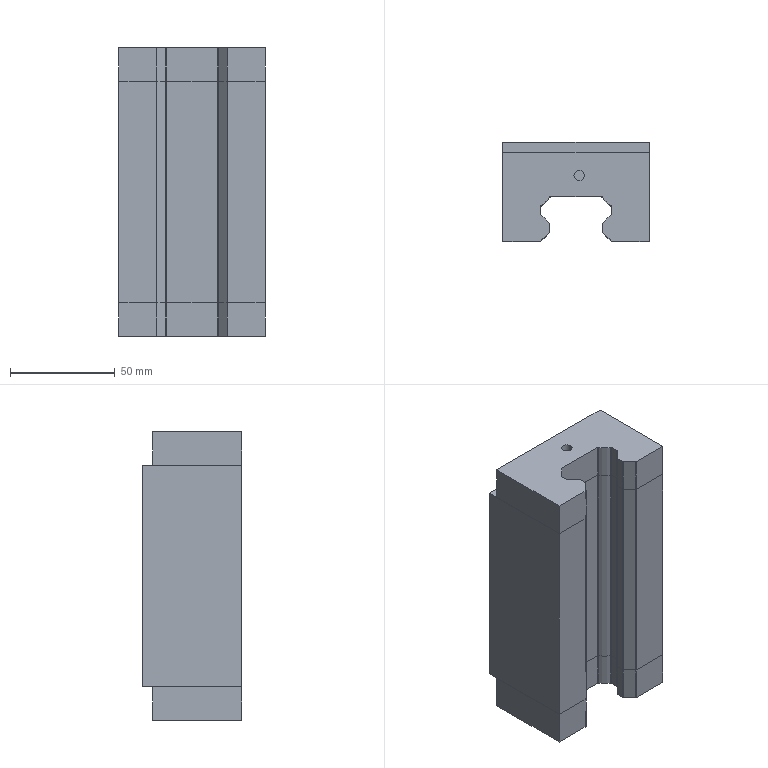Part | STEP file | HWH35HA Slider Block | 3 solids | 112 faces | box 70 x 47.5 x 138.2 mm | volume 358074 mm3 | cylinder 54 | plane 50 | cone 8 | commonest cylinder face diameters 1 x36 6.8 x8 18 x6 5 x4